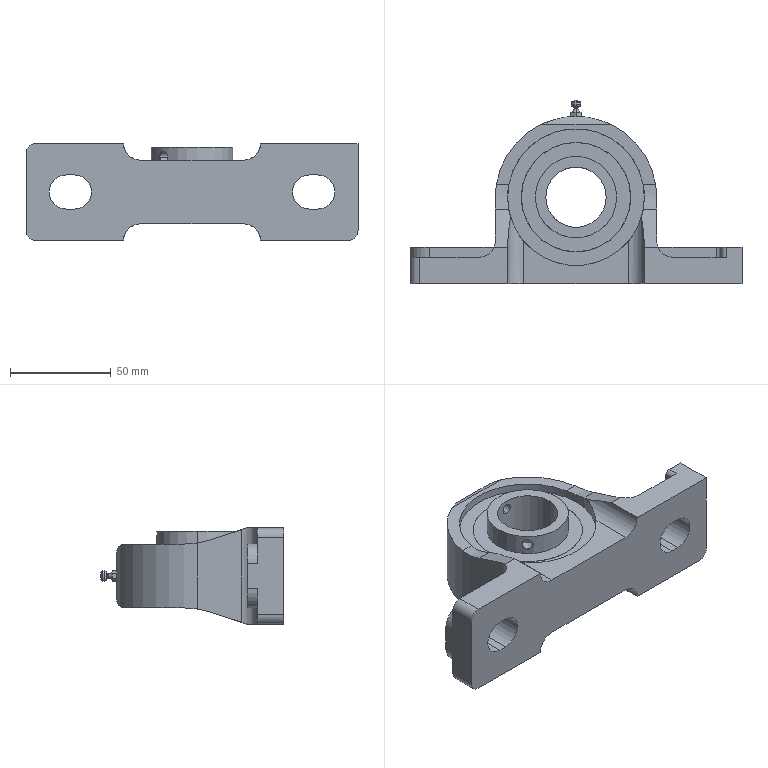Part | STEP file | PDR30_part | 1 solid | 112 faces | box 165 x 91 x 48 mm | volume 216054 mm3 | plane 49 | cylinder 43 | torus 12 | cone 6 | other 2 | commonest cylinder face diameters 16 x6 5.188 x4 17 x4 40.5 x4 68 x4 80 x4